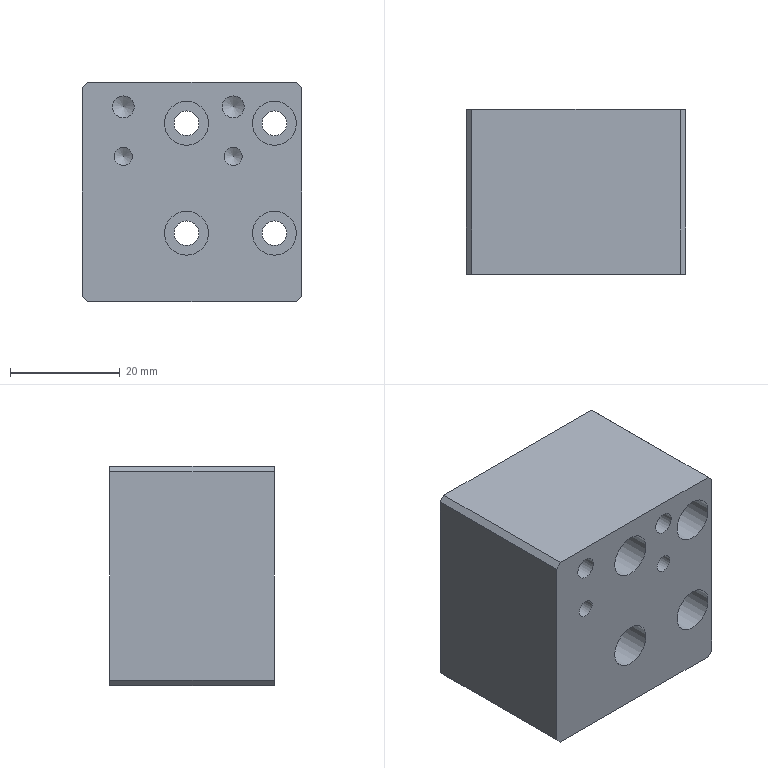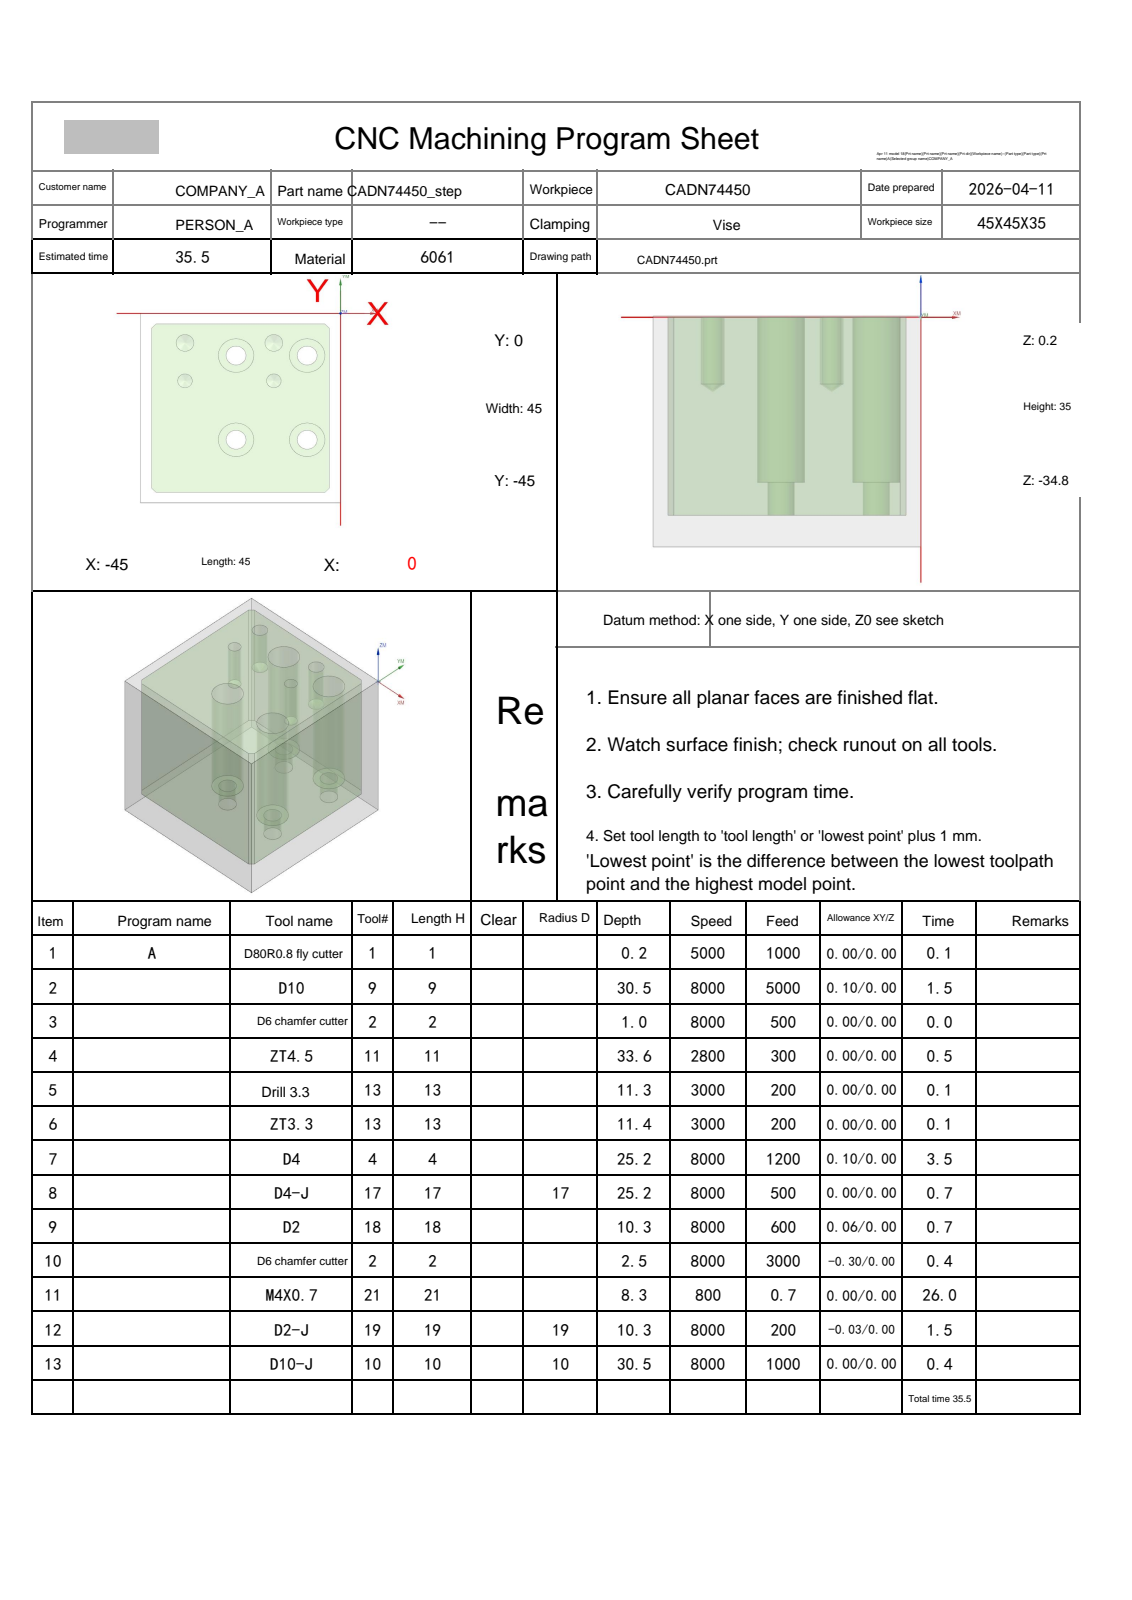NC program | NX | posted by the shop | part box 40 x 30 x 40 mm
Whole program, first 1137 of 1731 lines:
%
O0001
(Machine time: 61.34 MIN)
(===Total Tool:11===)
(T1=D80R0.8 fly cutter D=80.  R=0.8  D-  H01 Z=0.    )
(T9=D10     D=10.  R=0.   D-  H09 Z=-30.3 )
(T2=D6 chamfer cutter   D=6.   R=0.   D-  H02 Z=-2.3  )
(T11=ZT4.5  D=4.5  DR_a=118 D-  H11 Z=-33.35)
(T13=Drill 3.3  D=3.3  DR_a=118 D-  H13 Z=-11.2 )
(T4=D4      D=4.   R=0.   D-  H04 Z=-25.  )
(T17=D4-J   D=4.   R=0.   D17 H17 Z=-25.  )
(T18=D2     D=2.   R=0.   D-  H18 Z=-10.1 )
(T21=M4X0.7 D=3.3  DR_a=180 D-  H21 Z=-8.1  )
(T19=D2-J   D=2.   R=0.   D19 H19 Z=-10.1 )
(T10=D10-J  D=10.  R=0.   D10 H10 Z=-30.3 )
G80 G90 G17 G49 G40
G91 G28 Z0
M01
N1 T01 M06
(D80R0.8 fly cutter  D=80. R=0.8 H=01 ce=0.00 di=0.00)
G00 G90 G54 X-22.5 Y-87.5 M03 S5000
G43 H01 Z20.
M08
Z2.
G01 Z0.0 F1000.
Y-82.5
Y37.5
Y42.5
Z2.
G00 Z20.
G91 G28 Z0.0
M05
M09
G91 G28 Z0.0
M01
N2 T09 M06
(D10  D=10. R=0. H=09 ce=0.10 di=0.00)
G00 G90 G54 X-22.5 Y-47.6 M03 S8000
G43 H09 Z20.
M08
Z.5
G01 X-41.5 Z.421 F5000.
G02 X-45.106 Y-46.106 Z.404 I0.0 J5.1
G01 X-46.106 Y-45.106 Z.398
G02 X-47.6 Y-41.5 Z.382 I3.606 J3.606
G01 Y-3.5 Z.223
G02 X-46.106 Y.106 Z.207 I5.1 J0.0
G01 X-45.106 Y1.106 Z.201
G02 X-41.5 Y2.6 Z.184 I3.606 J-3.606
G01 X-3.5 Z.026
G02 X.106 Y1.106 Z.009 I0.0 J-5.1
G01 X1.106 Y.106 Z.003
G02 X2.6 Y-3.5 Z-.013 I-3.606 J-3.606
G01 Y-41.5 Z-.171
G02 X1.106 Y-45.106 Z-.188 I-5.1 J0.0
G01 X.106 Y-46.106 Z-.194
G02 X-3.5 Y-47.6 Z-.211 I-3.606 J3.606
G01 X-41.5 Z-.369
G02 X-45.106 Y-46.106 Z-.386 I0.0 J5.1
G01 X-46.106 Y-45.106 Z-.391
G02 X-47.6 Y-41.5 Z-.408 I3.606 J3.606
G01 Y-3.5 Z-.566
G02 X-46.106 Y.106 Z-.583 I5.1 J0.0
G01 X-45.106 Y1.106 Z-.589
G02 X-41.5 Y2.6 Z-.606 I3.606 J-3.606
G01 X-3.5 Z-.764
G02 X.106 Y1.106 Z-.78 I0.0 J-5.1
G01 X1.106 Y.106 Z-.786
G02 X2.6 Y-3.5 Z-.803 I-3.606 J-3.606
G01 Y-41.5 Z-.961
G02 X1.106 Y-45.106 Z-.978 I-5.1 J0.0
G01 X.106 Y-46.106 Z-.984
G02 X-3.5 Y-47.6 Z-1. I-3.606 J3.606
G01 X-41.5 Z-1.159
G02 X-45.106 Y-46.106 Z-1.175 I0.0 J5.1
G01 X-46.106 Y-45.106 Z-1.181
G02 X-47.6 Y-41.5 Z-1.198 I3.606 J3.606
G01 Y-3.5 Z-1.356
G02 X-46.106 Y.106 Z-1.373 I5.1 J0.0
G01 X-45.106 Y1.106 Z-1.379
G02 X-41.5 Y2.6 Z-1.395 I3.606 J-3.606
G01 X-3.5 Z-1.553
G02 X.106 Y1.106 Z-1.57 I0.0 J-5.1
G01 X1.106 Y.106 Z-1.576
G02 X2.6 Y-3.5 Z-1.593 I-3.606 J-3.606
G01 Y-41.5 Z-1.751
G02 X1.106 Y-45.106 Z-1.768 I-5.1 J0.0
G01 X.106 Y-46.106 Z-1.773
G02 X-3.5 Y-47.6 Z-1.79 I-3.606 J3.606
G01 X-41.5 Z-1.948
G02 X-45.106 Y-46.106 Z-1.965 I0.0 J5.1
G01 X-46.106 Y-45.106 Z-1.971
G02 X-47.6 Y-41.5 Z-1.988 I3.606 J3.606
G01 Y-3.5 Z-2.146
G02 X-46.106 Y.106 Z-2.162 I5.1 J0.0
G01 X-45.106 Y1.106 Z-2.168
G02 X-41.5 Y2.6 Z-2.185 I3.606 J-3.606
G01 X-3.5 Z-2.343
G02 X.106 Y1.106 Z-2.36 I0.0 J-5.1
G01 X1.106 Y.106 Z-2.366
G02 X2.6 Y-3.5 Z-2.382 I-3.606 J-3.606
G01 Y-41.5 Z-2.541
G02 X1.106 Y-45.106 Z-2.557 I-5.1 J0.0
G01 X.106 Y-46.106 Z-2.563
G02 X-3.5 Y-47.6 Z-2.58 I-3.606 J3.606
G01 X-41.5 Z-2.738
G02 X-45.106 Y-46.106 Z-2.755 I0.0 J5.1
G01 X-46.106 Y-45.106 Z-2.761
G02 X-47.6 Y-41.5 Z-2.777 I3.606 J3.606
G01 Y-3.5 Z-2.936
G02 X-46.106 Y.106 Z-2.952 I5.1 J0.0
G01 X-45.106 Y1.106 Z-2.958
G02 X-41.5 Y2.6 Z-2.975 I3.606 J-3.606
G01 X-3.5 Z-3.133
G02 X.106 Y1.106 Z-3.15 I0.0 J-5.1
G01 X1.106 Y.106 Z-3.156
G02 X2.6 Y-3.5 Z-3.172 I-3.606 J-3.606
G01 Y-41.5 Z-3.33
G02 X1.106 Y-45.106 Z-3.347 I-5.1 J0.0
G01 X.106 Y-46.106 Z-3.353
G02 X-3.5 Y-47.6 Z-3.37 I-3.606 J3.606
G01 X-41.5 Z-3.528
G02 X-45.106 Y-46.106 Z-3.544 I0.0 J5.1
G01 X-46.106 Y-45.106 Z-3.55
G02 X-47.6 Y-41.5 Z-3.567 I3.606 J3.606
G01 Y-3.5 Z-3.725
G02 X-46.106 Y.106 Z-3.742 I5.1 J0.0
G01 X-45.106 Y1.106 Z-3.748
G02 X-41.5 Y2.6 Z-3.764 I3.606 J-3.606
G01 X-3.5 Z-3.923
G02 X.106 Y1.106 Z-3.939 I0.0 J-5.1
G01 X1.106 Y.106 Z-3.945
G02 X2.6 Y-3.5 Z-3.962 I-3.606 J-3.606
G01 Y-41.5 Z-4.12
G02 X1.106 Y-45.106 Z-4.137 I-5.1 J0.0
G01 X.106 Y-46.106 Z-4.143
G02 X-3.5 Y-47.6 Z-4.159 I-3.606 J3.606
G01 X-41.5 Z-4.318
G02 X-45.106 Y-46.106 Z-4.334 I0.0 J5.1
G01 X-46.106 Y-45.106 Z-4.34
G02 X-47.6 Y-41.5 Z-4.357 I3.606 J3.606
G01 Y-3.5 Z-4.515
G02 X-46.106 Y.106 Z-4.532 I5.1 J0.0
G01 X-45.106 Y1.106 Z-4.538
G02 X-41.5 Y2.6 Z-4.554 I3.606 J-3.606
G01 X-3.5 Z-4.712
G02 X.106 Y1.106 Z-4.729 I0.0 J-5.1
G01 X1.106 Y.106 Z-4.735
G02 X2.6 Y-3.5 Z-4.752 I-3.606 J-3.606
G01 Y-41.5 Z-4.91
G02 X1.106 Y-45.106 Z-4.927 I-5.1 J0.0
G01 X.106 Y-46.106 Z-4.932
G02 X-3.5 Y-47.6 Z-4.949 I-3.606 J3.606
G01 X-41.5 Z-5.107
G02 X-45.106 Y-46.106 Z-5.124 I0.0 J5.1
G01 X-46.106 Y-45.106 Z-5.13
G02 X-47.6 Y-41.5 Z-5.147 I3.606 J3.606
G01 Y-3.5 Z-5.305
G02 X-46.106 Y.106 Z-5.321 I5.1 J0.0
G01 X-45.106 Y1.106 Z-5.327
G02 X-41.5 Y2.6 Z-5.344 I3.606 J-3.606
G01 X-3.5 Z-5.502
G02 X.106 Y1.106 Z-5.519 I0.0 J-5.1
G01 X1.106 Y.106 Z-5.525
G02 X2.6 Y-3.5 Z-5.541 I-3.606 J-3.606
G01 Y-41.5 Z-5.7
G02 X1.106 Y-45.106 Z-5.716 I-5.1 J0.0
G01 X.106 Y-46.106 Z-5.722
G02 X-3.5 Y-47.6 Z-5.739 I-3.606 J3.606
G01 X-41.5 Z-5.897
G02 X-45.106 Y-46.106 Z-5.914 I0.0 J5.1
G01 X-46.106 Y-45.106 Z-5.92
G02 X-47.6 Y-41.5 Z-5.936 I3.606 J3.606
G01 Y-3.5 Z-6.094
G02 X-46.106 Y.106 Z-6.111 I5.1 J0.0
G01 X-45.106 Y1.106 Z-6.117
G02 X-41.5 Y2.6 Z-6.134 I3.606 J-3.606
G01 X-3.5 Z-6.292
G02 X.106 Y1.106 Z-6.309 I0.0 J-5.1
G01 X1.106 Y.106 Z-6.314
G02 X2.6 Y-3.5 Z-6.331 I-3.606 J-3.606
G01 Y-41.5 Z-6.489
G02 X1.106 Y-45.106 Z-6.506 I-5.1 J0.0
G01 X.106 Y-46.106 Z-6.512
G02 X-3.5 Y-47.6 Z-6.529 I-3.606 J3.606
G01 X-41.5 Z-6.687
G02 X-45.106 Y-46.106 Z-6.703 I0.0 J5.1
G01 X-46.106 Y-45.106 Z-6.709
G02 X-47.6 Y-41.5 Z-6.726 I3.606 J3.606
G01 Y-3.5 Z-6.884
G02 X-46.106 Y.106 Z-6.901 I5.1 J0.0
G01 X-45.106 Y1.106 Z-6.907
G02 X-41.5 Y2.6 Z-6.923 I3.606 J-3.606
G01 X-3.5 Z-7.082
G02 X.106 Y1.106 Z-7.098 I0.0 J-5.1
G01 X1.106 Y.106 Z-7.104
G02 X2.6 Y-3.5 Z-7.121 I-3.606 J-3.606
G01 Y-41.5 Z-7.279
G02 X1.106 Y-45.106 Z-7.296 I-5.1 J0.0
G01 X.106 Y-46.106 Z-7.302
G02 X-3.5 Y-47.6 Z-7.318 I-3.606 J3.606
G01 X-41.5 Z-7.477
G02 X-45.106 Y-46.106 Z-7.493 I0.0 J5.1
G01 X-46.106 Y-45.106 Z-7.499
G02 X-47.6 Y-41.5 Z-7.516 I3.606 J3.606
G01 Y-3.5 Z-7.674
G02 X-46.106 Y.106 Z-7.691 I5.1 J0.0
G01 X-45.106 Y1.106 Z-7.697
G02 X-41.5 Y2.6 Z-7.713 I3.606 J-3.606
G01 X-3.5 Z-7.871
G02 X.106 Y1.106 Z-7.888 I0.0 J-5.1
G01 X1.106 Y.106 Z-7.894
G02 X2.6 Y-3.5 Z-7.911 I-3.606 J-3.606
G01 Y-41.5 Z-8.069
G02 X1.106 Y-45.106 Z-8.086 I-5.1 J0.0
G01 X.106 Y-46.106 Z-8.091
G02 X-3.5 Y-47.6 Z-8.108 I-3.606 J3.606
G01 X-41.5 Z-8.266
G02 X-45.106 Y-46.106 Z-8.283 I0.0 J5.1
G01 X-46.106 Y-45.106 Z-8.289
G02 X-47.6 Y-41.5 Z-8.306 I3.606 J3.606
G01 Y-3.5 Z-8.464
G02 X-46.106 Y.106 Z-8.48 I5.1 J0.0
G01 X-45.106 Y1.106 Z-8.486
G02 X-41.5 Y2.6 Z-8.503 I3.606 J-3.606
G01 X-3.5 Z-8.661
G02 X.106 Y1.106 Z-8.678 I0.0 J-5.1
G01 X1.106 Y.106 Z-8.684
G02 X2.6 Y-3.5 Z-8.7 I-3.606 J-3.606
G01 Y-41.5 Z-8.859
G02 X1.106 Y-45.106 Z-8.875 I-5.1 J0.0
G01 X.106 Y-46.106 Z-8.881
G02 X-3.5 Y-47.6 Z-8.898 I-3.606 J3.606
G01 X-41.5 Z-9.056
G02 X-45.106 Y-46.106 Z-9.073 I0.0 J5.1
G01 X-46.106 Y-45.106 Z-9.079
G02 X-47.6 Y-41.5 Z-9.095 I3.606 J3.606
G01 Y-3.5 Z-9.253
G02 X-46.106 Y.106 Z-9.27 I5.1 J0.0
G01 X-45.106 Y1.106 Z-9.276
G02 X-41.5 Y2.6 Z-9.293 I3.606 J-3.606
G01 X-3.5 Z-9.451
G02 X.106 Y1.106 Z-9.468 I0.0 J-5.1
G01 X1.106 Y.106 Z-9.473
G02 X2.6 Y-3.5 Z-9.49 I-3.606 J-3.606
G01 Y-41.5 Z-9.648
G02 X1.106 Y-45.106 Z-9.665 I-5.1 J0.0
G01 X.106 Y-46.106 Z-9.671
G02 X-3.5 Y-47.6 Z-9.688 I-3.606 J3.606
G01 X-41.5 Z-9.846
G02 X-45.106 Y-46.106 Z-9.862 I0.0 J5.1
G01 X-46.106 Y-45.106 Z-9.868
G02 X-47.6 Y-41.5 Z-9.885 I3.606 J3.606
G01 Y-3.5 Z-10.043
G02 X-46.106 Y.106 Z-10.06 I5.1 J0.0
G01 X-45.106 Y1.106 Z-10.066
G02 X-41.5 Y2.6 Z-10.082 I3.606 J-3.606
G01 X-3.5 Z-10.241
G02 X.106 Y1.106 Z-10.257 I0.0 J-5.1
G01 X1.106 Y.106 Z-10.263
G02 X2.6 Y-3.5 Z-10.28 I-3.606 J-3.606
G01 Y-41.5 Z-10.438
G02 X1.106 Y-45.106 Z-10.455 I-5.1 J0.0
G01 X.106 Y-46.106 Z-10.461
G02 X-3.5 Y-47.6 Z-10.477 I-3.606 J3.606
G01 X-41.5 Z-10.636
G02 X-45.106 Y-46.106 Z-10.652 I0.0 J5.1
G01 X-46.106 Y-45.106 Z-10.658
G02 X-47.6 Y-41.5 Z-10.675 I3.606 J3.606
G01 Y-3.5 Z-10.833
G02 X-46.106 Y.106 Z-10.85 I5.1 J0.0
G01 X-45.106 Y1.106 Z-10.856
G02 X-41.5 Y2.6 Z-10.872 I3.606 J-3.606
G01 X-3.5 Z-11.03
G02 X.106 Y1.106 Z-11.047 I0.0 J-5.1
G01 X1.106 Y.106 Z-11.053
G02 X2.6 Y-3.5 Z-11.07 I-3.606 J-3.606
G01 Y-41.5 Z-11.228
G02 X1.106 Y-45.106 Z-11.244 I-5.1 J0.0
G01 X.106 Y-46.106 Z-11.25
G02 X-3.5 Y-47.6 Z-11.267 I-3.606 J3.606
G01 X-41.5 Z-11.425
G02 X-45.106 Y-46.106 Z-11.442 I0.0 J5.1
G01 X-46.106 Y-45.106 Z-11.448
G02 X-47.6 Y-41.5 Z-11.464 I3.606 J3.606
G01 Y-3.5 Z-11.623
G02 X-46.106 Y.106 Z-11.639 I5.1 J0.0
G01 X-45.106 Y1.106 Z-11.645
G02 X-41.5 Y2.6 Z-11.662 I3.606 J-3.606
G01 X-3.5 Z-11.82
G02 X.106 Y1.106 Z-11.837 I0.0 J-5.1
G01 X1.106 Y.106 Z-11.843
G02 X2.6 Y-3.5 Z-11.859 I-3.606 J-3.606
G01 Y-41.5 Z-12.018
G02 X1.106 Y-45.106 Z-12.034 I-5.1 J0.0
G01 X.106 Y-46.106 Z-12.04
G02 X-3.5 Y-47.6 Z-12.057 I-3.606 J3.606
G01 X-41.5 Z-12.215
G02 X-45.106 Y-46.106 Z-12.232 I0.0 J5.1
G01 X-46.106 Y-45.106 Z-12.238
G02 X-47.6 Y-41.5 Z-12.254 I3.606 J3.606
G01 Y-3.5 Z-12.412
G02 X-46.106 Y.106 Z-12.429 I5.1 J0.0
G01 X-45.106 Y1.106 Z-12.435
G02 X-41.5 Y2.6 Z-12.452 I3.606 J-3.606
G01 X-3.5 Z-12.61
G02 X.106 Y1.106 Z-12.627 I0.0 J-5.1
G01 X1.106 Y.106 Z-12.632
G02 X2.6 Y-3.5 Z-12.649 I-3.606 J-3.606
G01 Y-41.5 Z-12.807
G02 X1.106 Y-45.106 Z-12.824 I-5.1 J0.0
G01 X.106 Y-46.106 Z-12.83
G02 X-3.5 Y-47.6 Z-12.847 I-3.606 J3.606
G01 X-41.5 Z-13.005
G02 X-45.106 Y-46.106 Z-13.021 I0.0 J5.1
G01 X-46.106 Y-45.106 Z-13.027
G02 X-47.6 Y-41.5 Z-13.044 I3.606 J3.606
G01 Y-3.5 Z-13.202
G02 X-46.106 Y.106 Z-13.219 I5.1 J0.0
G01 X-45.106 Y1.106 Z-13.225
G02 X-41.5 Y2.6 Z-13.241 I3.606 J-3.606
G01 X-3.5 Z-13.4
G02 X.106 Y1.106 Z-13.416 I0.0 J-5.1
G01 X1.106 Y.106 Z-13.422
G02 X2.6 Y-3.5 Z-13.439 I-3.606 J-3.606
G01 Y-41.5 Z-13.597
G02 X1.106 Y-45.106 Z-13.614 I-5.1 J0.0
G01 X.106 Y-46.106 Z-13.62
G02 X-3.5 Y-47.6 Z-13.636 I-3.606 J3.606
G01 X-41.5 Z-13.794
G02 X-45.106 Y-46.106 Z-13.811 I0.0 J5.1
G01 X-46.106 Y-45.106 Z-13.817
G02 X-47.6 Y-41.5 Z-13.834 I3.606 J3.606
G01 Y-3.5 Z-13.992
G02 X-46.106 Y.106 Z-14.009 I5.1 J0.0
G01 X-45.106 Y1.106 Z-14.014
G02 X-41.5 Y2.6 Z-14.031 I3.606 J-3.606
G01 X-3.5 Z-14.189
G02 X.106 Y1.106 Z-14.206 I0.0 J-5.1
G01 X1.106 Y.106 Z-14.212
G02 X2.6 Y-3.5 Z-14.229 I-3.606 J-3.606
G01 Y-41.5 Z-14.387
G02 X1.106 Y-45.106 Z-14.403 I-5.1 J0.0
G01 X.106 Y-46.106 Z-14.409
G02 X-3.5 Y-47.6 Z-14.426 I-3.606 J3.606
G01 X-41.5 Z-14.584
G02 X-45.106 Y-46.106 Z-14.601 I0.0 J5.1
G01 X-46.106 Y-45.106 Z-14.607
G02 X-47.6 Y-41.5 Z-14.623 I3.606 J3.606
G01 Y-3.5 Z-14.782
G02 X-46.106 Y.106 Z-14.798 I5.1 J0.0
G01 X-45.106 Y1.106 Z-14.804
G02 X-41.5 Y2.6 Z-14.821 I3.606 J-3.606
G01 X-3.5 Z-14.979
G02 X.106 Y1.106 Z-14.996 I0.0 J-5.1
G01 X1.106 Y.106 Z-15.002
G02 X2.6 Y-3.5 Z-15.018 I-3.606 J-3.606
G01 Y-41.5 Z-15.177
G02 X1.106 Y-45.106 Z-15.193 I-5.1 J0.0
G01 X.106 Y-46.106 Z-15.199
G02 X-3.5 Y-47.6 Z-15.216 I-3.606 J3.606
G01 X-41.5 Z-15.374
G02 X-45.106 Y-46.106 Z-15.391 I0.0 J5.1
G01 X-46.106 Y-45.106 Z-15.397
G02 X-47.6 Y-41.5 Z-15.413 I3.606 J3.606
G01 Y-3.5 Z-15.571
G02 X-46.106 Y.106 Z-15.588 I5.1 J0.0
G01 X-45.106 Y1.106 Z-15.594
G02 X-41.5 Y2.6 Z-15.611 I3.606 J-3.606
G01 X-3.5 Z-15.769
G02 X.106 Y1.106 Z-15.786 I0.0 J-5.1
G01 X1.106 Y.106 Z-15.791
G02 X2.6 Y-3.5 Z-15.808 I-3.606 J-3.606
G01 Y-41.5 Z-15.966
G02 X1.106 Y-45.106 Z-15.983 I-5.1 J0.0
G01 X.106 Y-46.106 Z-15.989
G02 X-3.5 Y-47.6 Z-16.006 I-3.606 J3.606
G01 X-41.5 Z-16.164
G02 X-45.106 Y-46.106 Z-16.18 I0.0 J5.1
G01 X-46.106 Y-45.106 Z-16.186
G02 X-47.6 Y-41.5 Z-16.203 I3.606 J3.606
G01 Y-3.5 Z-16.361
G02 X-46.106 Y.106 Z-16.378 I5.1 J0.0
G01 X-45.106 Y1.106 Z-16.384
G02 X-41.5 Y2.6 Z-16.4 I3.606 J-3.606
G01 X-3.5 Z-16.559
G02 X.106 Y1.106 Z-16.575 I0.0 J-5.1
G01 X1.106 Y.106 Z-16.581
G02 X2.6 Y-3.5 Z-16.598 I-3.606 J-3.606
G01 Y-41.5 Z-16.756
G02 X1.106 Y-45.106 Z-16.773 I-5.1 J0.0
G01 X.106 Y-46.106 Z-16.779
G02 X-3.5 Y-47.6 Z-16.795 I-3.606 J3.606
G01 X-41.5 Z-16.953
G02 X-45.106 Y-46.106 Z-16.97 I0.0 J5.1
G01 X-46.106 Y-45.106 Z-16.976
G02 X-47.6 Y-41.5 Z-16.993 I3.606 J3.606
G01 Y-3.5 Z-17.151
G02 X-46.106 Y.106 Z-17.168 I5.1 J0.0
G01 X-45.106 Y1.106 Z-17.173
G02 X-41.5 Y2.6 Z-17.19 I3.606 J-3.606
G01 X-3.5 Z-17.348
G02 X.106 Y1.106 Z-17.365 I0.0 J-5.1
G01 X1.106 Y.106 Z-17.371
G02 X2.6 Y-3.5 Z-17.388 I-3.606 J-3.606
G01 Y-41.5 Z-17.546
G02 X1.106 Y-45.106 Z-17.562 I-5.1 J0.0
G01 X.106 Y-46.106 Z-17.568
G02 X-3.5 Y-47.6 Z-17.585 I-3.606 J3.606
G01 X-41.5 Z-17.743
G02 X-45.106 Y-46.106 Z-17.76 I0.0 J5.1
G01 X-46.106 Y-45.106 Z-17.766
G02 X-47.6 Y-41.5 Z-17.782 I3.606 J3.606
G01 Y-3.5 Z-17.941
G02 X-46.106 Y.106 Z-17.957 I5.1 J0.0
G01 X-45.106 Y1.106 Z-17.963
G02 X-41.5 Y2.6 Z-17.98 I3.606 J-3.606
G01 X-3.5 Z-18.138
G02 X.106 Y1.106 Z-18.155 I0.0 J-5.1
G01 X1.106 Y.106 Z-18.161
G02 X2.6 Y-3.5 Z-18.177 I-3.606 J-3.606
G01 Y-41.5 Z-18.336
G02 X1.106 Y-45.106 Z-18.352 I-5.1 J0.0
G01 X.106 Y-46.106 Z-18.358
G02 X-3.5 Y-47.6 Z-18.375 I-3.606 J3.606
G01 X-41.5 Z-18.533
G02 X-45.106 Y-46.106 Z-18.55 I0.0 J5.1
G01 X-46.106 Y-45.106 Z-18.556
G02 X-47.6 Y-41.5 Z-18.572 I3.606 J3.606
G01 Y-3.5 Z-18.73
G02 X-46.106 Y.106 Z-18.747 I5.1 J0.0
G01 X-45.106 Y1.106 Z-18.753
G02 X-41.5 Y2.6 Z-18.77 I3.606 J-3.606
G01 X-3.5 Z-18.928
G02 X.106 Y1.106 Z-18.944 I0.0 J-5.1
G01 X1.106 Y.106 Z-18.95
G02 X2.6 Y-3.5 Z-18.967 I-3.606 J-3.606
G01 Y-41.5 Z-19.125
G02 X1.106 Y-45.106 Z-19.142 I-5.1 J0.0
G01 X.106 Y-46.106 Z-19.148
G02 X-3.5 Y-47.6 Z-19.164 I-3.606 J3.606
G01 X-41.5 Z-19.323
G02 X-45.106 Y-46.106 Z-19.339 I0.0 J5.1
G01 X-46.106 Y-45.106 Z-19.345
G02 X-47.6 Y-41.5 Z-19.362 I3.606 J3.606
G01 Y-3.5 Z-19.52
G02 X-46.106 Y.106 Z-19.537 I5.1 J0.0
G01 X-45.106 Y1.106 Z-19.543
G02 X-41.5 Y2.6 Z-19.559 I3.606 J-3.606
G01 X-3.5 Z-19.718
G02 X.106 Y1.106 Z-19.734 I0.0 J-5.1
G01 X1.106 Y.106 Z-19.74
G02 X2.6 Y-3.5 Z-19.757 I-3.606 J-3.606
G01 Y-41.5 Z-19.915
G02 X1.106 Y-45.106 Z-19.932 I-5.1 J0.0
G01 X.106 Y-46.106 Z-19.938
G02 X-3.5 Y-47.6 Z-19.954 I-3.606 J3.606
G01 X-41.5 Z-20.112
G02 X-45.106 Y-46.106 Z-20.129 I0.0 J5.1
G01 X-46.106 Y-45.106 Z-20.135
G02 X-47.6 Y-41.5 Z-20.152 I3.606 J3.606
G01 Y-3.5 Z-20.31
G02 X-46.106 Y.106 Z-20.327 I5.1 J0.0
G01 X-45.106 Y1.106 Z-20.332
G02 X-41.5 Y2.6 Z-20.349 I3.606 J-3.606
G01 X-3.5 Z-20.507
G02 X.106 Y1.106 Z-20.524 I0.0 J-5.1
G01 X1.106 Y.106 Z-20.53
G02 X2.6 Y-3.5 Z-20.547 I-3.606 J-3.606
G01 Y-41.5 Z-20.705
G02 X1.106 Y-45.106 Z-20.721 I-5.1 J0.0
G01 X.106 Y-46.106 Z-20.727
G02 X-3.5 Y-47.6 Z-20.744 I-3.606 J3.606
G01 X-41.5 Z-20.902
G02 X-45.106 Y-46.106 Z-20.919 I0.0 J5.1
G01 X-46.106 Y-45.106 Z-20.925
G02 X-47.6 Y-41.5 Z-20.941 I3.606 J3.606
G01 Y-3.5 Z-21.1
G02 X-46.106 Y.106 Z-21.116 I5.1 J0.0
G01 X-45.106 Y1.106 Z-21.122
G02 X-41.5 Y2.6 Z-21.139 I3.606 J-3.606
G01 X-3.5 Z-21.297
G02 X.106 Y1.106 Z-21.314 I0.0 J-5.1
G01 X1.106 Y.106 Z-21.32
G02 X2.6 Y-3.5 Z-21.336 I-3.606 J-3.606
G01 Y-41.5 Z-21.494
G02 X1.106 Y-45.106 Z-21.511 I-5.1 J0.0
G01 X.106 Y-46.106 Z-21.517
G02 X-3.5 Y-47.6 Z-21.534 I-3.606 J3.606
G01 X-41.5 Z-21.692
G02 X-45.106 Y-46.106 Z-21.709 I0.0 J5.1
G01 X-46.106 Y-45.106 Z-21.714
G02 X-47.6 Y-41.5 Z-21.731 I3.606 J3.606
G01 Y-3.5 Z-21.889
G02 X-46.106 Y.106 Z-21.906 I5.1 J0.0
G01 X-45.106 Y1.106 Z-21.912
G02 X-41.5 Y2.6 Z-21.929 I3.606 J-3.606
G01 X-3.5 Z-22.087
G02 X.106 Y1.106 Z-22.103 I0.0 J-5.1
G01 X1.106 Y.106 Z-22.109
G02 X2.6 Y-3.5 Z-22.126 I-3.606 J-3.606
G01 Y-41.5 Z-22.284
G02 X1.106 Y-45.106 Z-22.301 I-5.1 J0.0
G01 X.106 Y-46.106 Z-22.307
G02 X-3.5 Y-47.6 Z-22.323 I-3.606 J3.606
G01 X-41.5 Z-22.482
G02 X-45.106 Y-46.106 Z-22.498 I0.0 J5.1
G01 X-46.106 Y-45.106 Z-22.504
G02 X-47.6 Y-41.5 Z-22.521 I3.606 J3.606
G01 Y-3.5 Z-22.679
G02 X-46.106 Y.106 Z-22.696 I5.1 J0.0
G01 X-45.106 Y1.106 Z-22.702
G02 X-41.5 Y2.6 Z-22.718 I3.606 J-3.606
G01 X-3.5 Z-22.877
G02 X.106 Y1.106 Z-22.893 I0.0 J-5.1
G01 X1.106 Y.106 Z-22.899
G02 X2.6 Y-3.5 Z-22.916 I-3.606 J-3.606
G01 Y-41.5 Z-23.074
G02 X1.106 Y-45.106 Z-23.091 I-5.1 J0.0
G01 X.106 Y-46.106 Z-23.097
G02 X-3.5 Y-47.6 Z-23.113 I-3.606 J3.606
G01 X-41.5 Z-23.271
G02 X-45.106 Y-46.106 Z-23.288 I0.0 J5.1
G01 X-46.106 Y-45.106 Z-23.294
G02 X-47.6 Y-41.5 Z-23.311 I3.606 J3.606
G01 Y-3.5 Z-23.469
G02 X-46.106 Y.106 Z-23.486 I5.1 J0.0
G01 X-45.106 Y1.106 Z-23.491
G02 X-41.5 Y2.6 Z-23.508 I3.606 J-3.606
G01 X-3.5 Z-23.666
G02 X.106 Y1.106 Z-23.683 I0.0 J-5.1
G01 X1.106 Y.106 Z-23.689
G02 X2.6 Y-3.5 Z-23.706 I-3.606 J-3.606
G01 Y-41.5 Z-23.864
G02 X1.106 Y-45.106 Z-23.88 I-5.1 J0.0
G01 X.106 Y-46.106 Z-23.886
G02 X-3.5 Y-47.6 Z-23.903 I-3.606 J3.606
G01 X-41.5 Z-24.061
G02 X-45.106 Y-46.106 Z-24.078 I0.0 J5.1
G01 X-46.106 Y-45.106 Z-24.084
G02 X-47.6 Y-41.5 Z-24.1 I3.606 J3.606
G01 Y-3.5 Z-24.259
G02 X-46.106 Y.106 Z-24.275 I5.1 J0.0
G01 X-45.106 Y1.106 Z-24.281
G02 X-41.5 Y2.6 Z-24.298 I3.606 J-3.606
G01 X-3.5 Z-24.456
G02 X.106 Y1.106 Z-24.473 I0.0 J-5.1
G01 X1.106 Y.106 Z-24.479
G02 X2.6 Y-3.5 Z-24.495 I-3.606 J-3.606
G01 Y-41.5 Z-24.653
G02 X1.106 Y-45.106 Z-24.67 I-5.1 J0.0
G01 X.106 Y-46.106 Z-24.676
G02 X-3.5 Y-47.6 Z-24.693 I-3.606 J3.606
G01 X-41.5 Z-24.851
G02 X-45.106 Y-46.106 Z-24.868 I0.0 J5.1
G01 X-46.106 Y-45.106 Z-24.873
G02 X-47.6 Y-41.5 Z-24.89 I3.606 J3.606
G01 Y-3.5 Z-25.048
G02 X-46.106 Y.106 Z-25.065 I5.1 J0.0
G01 X-45.106 Y1.106 Z-25.071
G02 X-41.5 Y2.6 Z-25.088 I3.606 J-3.606
G01 X-3.5 Z-25.246
G02 X.106 Y1.106 Z-25.262 I0.0 J-5.1
G01 X1.106 Y.106 Z-25.268
G02 X2.6 Y-3.5 Z-25.285 I-3.606 J-3.606
G01 Y-41.5 Z-25.443
G02 X1.106 Y-45.106 Z-25.46 I-5.1 J0.0
G01 X.106 Y-46.106 Z-25.466
G02 X-3.5 Y-47.6 Z-25.482 I-3.606 J3.606
G01 X-41.5 Z-25.641
G02 X-45.106 Y-46.106 Z-25.657 I0.0 J5.1
G01 X-46.106 Y-45.106 Z-25.663
G02 X-47.6 Y-41.5 Z-25.68 I3.606 J3.606
G01 Y-3.5 Z-25.838
G02 X-46.106 Y.106 Z-25.855 I5.1 J0.0
G01 X-45.106 Y1.106 Z-25.861
G02 X-41.5 Y2.6 Z-25.877 I3.606 J-3.606
G01 X-3.5 Z-26.036
G02 X.106 Y1.106 Z-26.052 I0.0 J-5.1
G01 X1.106 Y.106 Z-26.058
G02 X2.6 Y-3.5 Z-26.075 I-3.606 J-3.606
G01 Y-41.5 Z-26.233
G02 X1.106 Y-45.106 Z-26.25 I-5.1 J0.0
G01 X.106 Y-46.106 Z-26.256
G02 X-3.5 Y-47.6 Z-26.272 I-3.606 J3.606
G01 X-41.5 Z-26.43
G02 X-45.106 Y-46.106 Z-26.447 I0.0 J5.1
G01 X-46.106 Y-45.106 Z-26.453
G02 X-47.6 Y-41.5 Z-26.47 I3.606 J3.606
G01 Y-3.5 Z-26.628
G02 X-46.106 Y.106 Z-26.644 I5.1 J0.0
G01 X-45.106 Y1.106 Z-26.65
G02 X-41.5 Y2.6 Z-26.667 I3.606 J-3.606
G01 X-3.5 Z-26.825
G02 X.106 Y1.106 Z-26.842 I0.0 J-5.1
G01 X1.106 Y.106 Z-26.848
G02 X2.6 Y-3.5 Z-26.864 I-3.606 J-3.606
G01 Y-41.5 Z-27.023
G02 X1.106 Y-45.106 Z-27.039 I-5.1 J0.0
G01 X.106 Y-46.106 Z-27.045
G02 X-3.5 Y-47.6 Z-27.062 I-3.606 J3.606
G01 X-41.5 Z-27.22
G02 X-45.106 Y-46.106 Z-27.237 I0.0 J5.1
G01 X-46.106 Y-45.106 Z-27.243
G02 X-47.6 Y-41.5 Z-27.259 I3.606 J3.606
G01 Y-3.5 Z-27.418
G02 X-46.106 Y.106 Z-27.434 I5.1 J0.0
G01 X-45.106 Y1.106 Z-27.44
G02 X-41.5 Y2.6 Z-27.457 I3.606 J-3.606
G01 X-3.5 Z-27.615
G02 X.106 Y1.106 Z-27.632 I0.0 J-5.1
G01 X1.106 Y.106 Z-27.638
G02 X2.6 Y-3.5 Z-27.654 I-3.606 J-3.606
G01 Y-41.5 Z-27.812
G02 X1.106 Y-45.106 Z-27.829 I-5.1 J0.0
G01 X.106 Y-46.106 Z-27.835
G02 X-3.5 Y-47.6 Z-27.852 I-3.606 J3.606
G01 X-41.5 Z-28.01
G02 X-45.106 Y-46.106 Z-28.027 I0.0 J5.1
G01 X-46.106 Y-45.106 Z-28.032
G02 X-47.6 Y-41.5 Z-28.049 I3.606 J3.606
G01 Y-3.5 Z-28.207
G02 X-46.106 Y.106 Z-28.224 I5.1 J0.0
G01 X-45.106 Y1.106 Z-28.23
G02 X-41.5 Y2.6 Z-28.247 I3.606 J-3.606
G01 X-3.5 Z-28.405
G02 X.106 Y1.106 Z-28.421 I0.0 J-5.1
G01 X1.106 Y.106 Z-28.427
G02 X2.6 Y-3.5 Z-28.444 I-3.606 J-3.606
G01 Y-41.5 Z-28.602
G02 X1.106 Y-45.106 Z-28.619 I-5.1 J0.0
G01 X.106 Y-46.106 Z-28.625
G02 X-3.5 Y-47.6 Z-28.641 I-3.606 J3.606
G01 X-41.5 Z-28.8
G02 X-45.106 Y-46.106 Z-28.816 I0.0 J5.1
G01 X-46.106 Y-45.106 Z-28.822
G02 X-47.6 Y-41.5 Z-28.839 I3.606 J3.606
G01 Y-3.5 Z-28.997
G02 X-46.106 Y.106 Z-29.014 I5.1 J0.0
G01 X-45.106 Y1.106 Z-29.02
G02 X-41.5 Y2.6 Z-29.036 I3.606 J-3.606
G01 X-3.5 Z-29.194
G02 X.106 Y1.106 Z-29.211 I0.0 J-5.1
G01 X1.106 Y.106 Z-29.217
G02 X2.6 Y-3.5 Z-29.234 I-3.606 J-3.606
G01 Y-41.5 Z-29.392
G02 X1.106 Y-45.106 Z-29.409 I-5.1 J0.0
G01 X.106 Y-46.106 Z-29.414
G02 X-3.5 Y-47.6 Z-29.431 I-3.606 J3.606
G01 X-41.5 Z-29.589
G02 X-45.106 Y-46.106 Z-29.606 I0.0 J5.1
G01 X-46.106 Y-45.106 Z-29.612
G02 X-47.6 Y-41.5 Z-29.629 I3.606 J3.606
G01 Y-3.5 Z-29.787
G02 X-46.106 Y.106 Z-29.803 I5.1 J0.0
G01 X-45.106 Y1.106 Z-29.809
G02 X-41.5 Y2.6 Z-29.826 I3.606 J-3.606
G01 X-3.5 Z-29.984
G02 X.106 Y1.106 Z-30.001 I0.0 J-5.1
G01 X1.106 Y.106 Z-30.007
G02 X2.6 Y-3.5 Z-30.023 I-3.606 J-3.606
G01 Y-41.5 Z-30.182
G02 X1.106 Y-45.106 Z-30.198 I-5.1 J0.0
G01 X.106 Y-46.106 Z-30.204
G02 X-3.5 Y-47.6 Z-30.221 I-3.606 J3.606
G01 X-22.5 Z-30.3
X-41.5
G02 X-45.106 Y-46.106 I0.0 J5.1
G01 X-46.106 Y-45.106
G02 X-47.6 Y-41.5 I3.606 J3.606
G01 Y-3.5
G02 X-46.106 Y.106 I5.1 J0.0
G01 X-45.106 Y1.106
G02 X-41.5 Y2.6 I3.606 J-3.606
G01 X-3.5
G02 X.106 Y1.106 I0.0 J-5.1
G01 X1.106 Y.106
G02 X2.6 Y-3.5 I-3.606 J-3.606
G01 Y-41.5
G02 X1.106 Y-45.106 I-5.1 J0.0
G01 X.106 Y-46.106
G02 X-3.5 Y-47.6 I-3.606 J3.606
G01 X-22.5
X-23.
Z-29.3
G00 Z20.
G91 G28 Z0.0
M05
M09
G91 G28 Z0.0
M01
N3 T02 M06
(D6 chamfer cutter  D=6. R=0. H=02 ce=0.00 di=0.00)
G00 G90 G54 X-35. Y-16. M03 S8000
G43 H02 Z20.
M08
G98 G81 X-35. Y-16. Z-.8 R1. F500.
Y-7.
X-23.5 Y-10.
X-15. Y-7.
X-7.5 Y-10.
X-15. Y-16.
X-7.5 Y-30.
X-23.5
G80
G00 Z20.
G91 G28 Z0.0
M05
M09
G91 G28 Z0.0
M01
N4 T11 M06
(ZT4.5 D=4.5 DR_a=118 H=11)
G00 G90 G54 X-23.5 Y-30. M03 S2800
G43 H11 Z20.
M08
G98 G83 X-23.5 Y-30. Z-33.352 R1. F300. Q2.
X-7.5
Y-10.
X-23.5
G80
G00 Z20.
G91 G28 Z0.0
M05
M09
G91 G28 Z0.0
M01
N5 T13 M06
(Drill 3.3 D=3.3 DR_a=118 H=13)
G00 G90 G54 X-35. Y-16. M03 S3000
G43 H13 Z20.
M08
G98 G83 X-35. Y-16. Z-11.091 R1. F200. Q2.
X-15.
G80
G00 Z20.
G91 G28 Z0.0
M05
M09
G91 G28 Z0.0
M01
N6 T13 M06
(ZT3.3 D=3.3 DR_a=118 H=13)
G00 G90 G54 X-35. Y-7. M03 S3000
G43 H13 Z20.
M08
G98 G83 X-35. Y-7. Z-11.202 R1. F200. Q2.
X-15.
G80
G00 Z20.
G91 G28 Z0.0
M05
M09
G91 G28 Z0.0
M01
N7 T04 M06
(D4  D=4. R=0. H=04 ce=0.10 di=0.00)
G00 G90 G54 X-23.5 Y-30. M03 S8000
G43 H04 Z20.
M08
Z.5
G03 X-22.55 Y-30.95 I.95 J0.0 F1200.
X-21.6 Y-30. I0.0 J.95
X-21.6 Y-30. Z.2 I-1.9 J0.0
X-21.6 Y-30. Z-.1 I-1.9 J0.0
X-21.6 Y-30. Z-.4 I-1.9 J0.0
X-21.6 Y-30. Z-.7 I-1.9 J0.0
X-21.6 Y-30. Z-1. I-1.9 J0.0
X-21.6 Y-30. Z-1.3 I-1.9 J0.0
X-21.6 Y-30. Z-1.6 I-1.9 J0.0
X-21.6 Y-30. Z-1.9 I-1.9 J0.0
X-21.6 Y-30. Z-2.2 I-1.9 J0.0
X-21.6 Y-30. Z-2.5 I-1.9 J0.0
X-21.6 Y-30. Z-2.8 I-1.9 J0.0
X-21.6 Y-30. Z-3.1 I-1.9 J0.0
X-21.6 Y-30. Z-3.4 I-1.9 J0.0
X-21.6 Y-30. Z-3.7 I-1.9 J0.0
X-21.6 Y-30. Z-4. I-1.9 J0.0
X-21.6 Y-30. Z-4.3 I-1.9 J0.0
X-21.6 Y-30. Z-4.6 I-1.9 J0.0
X-21.6 Y-30. Z-4.9 I-1.9 J0.0
X-21.6 Y-30. Z-5.2 I-1.9 J0.0
X-21.6 Y-30. Z-5.5 I-1.9 J0.0
X-21.6 Y-30. Z-5.8 I-1.9 J0.0
X-21.6 Y-30. Z-6.1 I-1.9 J0.0
X-21.6 Y-30. Z-6.4 I-1.9 J0.0
X-21.6 Y-30. Z-6.7 I-1.9 J0.0
X-21.6 Y-30. Z-7. I-1.9 J0.0
X-21.6 Y-30. Z-7.3 I-1.9 J0.0
X-21.6 Y-30. Z-7.6 I-1.9 J0.0
X-21.6 Y-30. Z-7.9 I-1.9 J0.0
X-21.6 Y-30. Z-8.2 I-1.9 J0.0
X-21.6 Y-30. Z-8.5 I-1.9 J0.0
X-21.6 Y-30. Z-8.8 I-1.9 J0.0
X-21.6 Y-30. Z-9.1 I-1.9 J0.0
X-21.6 Y-30. Z-9.4 I-1.9 J0.0
X-21.6 Y-30. Z-9.7 I-1.9 J0.0
X-21.6 Y-30. Z-10. I-1.9 J0.0
X-21.6 Y-30. Z-10.3 I-1.9 J0.0
X-21.6 Y-30. Z-10.6 I-1.9 J0.0
X-21.6 Y-30. Z-10.9 I-1.9 J0.0
X-21.6 Y-30. Z-11.2 I-1.9 J0.0
X-21.6 Y-30. Z-11.5 I-1.9 J0.0
X-21.6 Y-30. Z-11.8 I-1.9 J0.0
X-21.6 Y-30. Z-12.1 I-1.9 J0.0
X-21.6 Y-30. Z-12.4 I-1.9 J0.0
X-21.6 Y-30. Z-12.7 I-1.9 J0.0
X-21.6 Y-30. Z-13. I-1.9 J0.0
X-21.6 Y-30. Z-13.3 I-1.9 J0.0
X-21.6 Y-30. Z-13.6 I-1.9 J0.0
X-21.6 Y-30. Z-13.9 I-1.9 J0.0
X-21.6 Y-30. Z-14.2 I-1.9 J0.0
X-21.6 Y-30. Z-14.5 I-1.9 J0.0
X-21.6 Y-30. Z-14.8 I-1.9 J0.0
X-21.6 Y-30. Z-15.1 I-1.9 J0.0
X-21.6 Y-30. Z-15.4 I-1.9 J0.0
X-21.6 Y-30. Z-15.7 I-1.9 J0.0
X-21.6 Y-30. Z-16. I-1.9 J0.0
X-21.6 Y-30. Z-16.3 I-1.9 J0.0
X-21.6 Y-30. Z-16.6 I-1.9 J0.0
X-21.6 Y-30. Z-16.9 I-1.9 J0.0
X-21.6 Y-30. Z-17.2 I-1.9 J0.0
X-21.6 Y-30. Z-17.5 I-1.9 J0.0
X-21.6 Y-30. Z-17.8 I-1.9 J0.0
X-21.6 Y-30. Z-18.1 I-1.9 J0.0
X-21.6 Y-30. Z-18.4 I-1.9 J0.0
X-21.6 Y-30. Z-18.7 I-1.9 J0.0
X-21.6 Y-30. Z-19. I-1.9 J0.0
X-21.6 Y-30. Z-19.3 I-1.9 J0.0
X-21.6 Y-30. Z-19.6 I-1.9 J0.0
X-21.6 Y-30. Z-19.9 I-1.9 J0.0
X-21.6 Y-30. Z-20.2 I-1.9 J0.0
X-21.6 Y-30. Z-20.5 I-1.9 J0.0
X-21.6 Y-30. Z-20.8 I-1.9 J0.0
X-21.6 Y-30. Z-21.1 I-1.9 J0.0
X-21.6 Y-30. Z-21.4 I-1.9 J0.0
X-21.6 Y-30. Z-21.7 I-1.9 J0.0
X-21.6 Y-30. Z-22. I-1.9 J0.0
X-21.6 Y-30. Z-22.3 I-1.9 J0.0
X-21.6 Y-30. Z-22.6 I-1.9 J0.0
X-21.6 Y-30. Z-22.9 I-1.9 J0.0
X-21.6 Y-30. Z-23.2 I-1.9 J0.0
X-21.6 Y-30. Z-23.5 I-1.9 J0.0
X-21.6 Y-30. Z-23.8 I-1.9 J0.0
X-21.6 Y-30. Z-24.1 I-1.9 J0.0
X-21.6 Y-30. Z-24.4 I-1.9 J0.0
X-21.6 Y-30. Z-24.7 I-1.9 J0.0
X-21.6 Y-30. Z-25. I-1.9 J0.0
X-23.5 Y-28.1 I-1.9 J0.0
X-25.4 Y-30. I0.0 J-1.9
X-23.5 Y-31.9 I1.9 J0.0
X-21.6 Y-30. I0.0 J1.9
X-22.55 Y-29.05 I-.95 J0.0
X-23.5 Y-30. I0.0 J-.95
G00 Z20.
X-7.5
Z.5
G03 X-6.55 Y-30.95 I.95 J0.0
X-5.6 Y-30. I0.0 J.95
X-5.6 Y-30. Z.2 I-1.9 J0.0
X-5.6 Y-30. Z-.1 I-1.9 J0.0
X-5.6 Y-30. Z-.4 I-1.9 J0.0
X-5.6 Y-30. Z-.7 I-1.9 J0.0
X-5.6 Y-30. Z-1. I-1.9 J0.0
X-5.6 Y-30. Z-1.3 I-1.9 J0.0
X-5.6 Y-30. Z-1.6 I-1.9 J0.0
X-5.6 Y-30. Z-1.9 I-1.9 J0.0
X-5.6 Y-30. Z-2.2 I-1.9 J0.0
X-5.6 Y-30. Z-2.5 I-1.9 J0.0
X-5.6 Y-30. Z-2.8 I-1.9 J0.0
X-5.6 Y-30. Z-3.1 I-1.9 J0.0
X-5.6 Y-30. Z-3.4 I-1.9 J0.0
X-5.6 Y-30. Z-3.7 I-1.9 J0.0
X-5.6 Y-30. Z-4. I-1.9 J0.0
X-5.6 Y-30. Z-4.3 I-1.9 J0.0
X-5.6 Y-30. Z-4.6 I-1.9 J0.0
X-5.6 Y-30. Z-4.9 I-1.9 J0.0
X-5.6 Y-30. Z-5.2 I-1.9 J0.0
X-5.6 Y-30. Z-5.5 I-1.9 J0.0
X-5.6 Y-30. Z-5.8 I-1.9 J0.0
X-5.6 Y-30. Z-6.1 I-1.9 J0.0
X-5.6 Y-30. Z-6.4 I-1.9 J0.0
X-5.6 Y-30. Z-6.7 I-1.9 J0.0
X-5.6 Y-30. Z-7. I-1.9 J0.0
X-5.6 Y-30. Z-7.3 I-1.9 J0.0
X-5.6 Y-30. Z-7.6 I-1.9 J0.0
X-5.6 Y-30. Z-7.9 I-1.9 J0.0
X-5.6 Y-30. Z-8.2 I-1.9 J0.0
X-5.6 Y-30. Z-8.5 I-1.9 J0.0
X-5.6 Y-30. Z-8.8 I-1.9 J0.0
X-5.6 Y-30. Z-9.1 I-1.9 J0.0
X-5.6 Y-30. Z-9.4 I-1.9 J0.0
X-5.6 Y-30. Z-9.7 I-1.9 J0.0
X-5.6 Y-30. Z-10. I-1.9 J0.0
X-5.6 Y-30. Z-10.3 I-1.9 J0.0
X-5.6 Y-30. Z-10.6 I-1.9 J0.0
X-5.6 Y-30. Z-10.9 I-1.9 J0.0
X-5.6 Y-30. Z-11.2 I-1.9 J0.0
X-5.6 Y-30. Z-11.5 I-1.9 J0.0
X-5.6 Y-30. Z-11.8 I-1.9 J0.0
X-5.6 Y-30. Z-12.1 I-1.9 J0.0
X-5.6 Y-30. Z-12.4 I-1.9 J0.0
X-5.6 Y-30. Z-12.7 I-1.9 J0.0
X-5.6 Y-30. Z-13. I-1.9 J0.0
X-5.6 Y-30. Z-13.3 I-1.9 J0.0
X-5.6 Y-30. Z-13.6 I-1.9 J0.0
X-5.6 Y-30. Z-13.9 I-1.9 J0.0
X-5.6 Y-30. Z-14.2 I-1.9 J0.0
X-5.6 Y-30. Z-14.5 I-1.9 J0.0
X-5.6 Y-30. Z-14.8 I-1.9 J0.0
X-5.6 Y-30. Z-15.1 I-1.9 J0.0
X-5.6 Y-30. Z-15.4 I-1.9 J0.0
X-5.6 Y-30. Z-15.7 I-1.9 J0.0
X-5.6 Y-30. Z-16. I-1.9 J0.0
X-5.6 Y-30. Z-16.3 I-1.9 J0.0
X-5.6 Y-30. Z-16.6 I-1.9 J0.0
X-5.6 Y-30. Z-16.9 I-1.9 J0.0
X-5.6 Y-30. Z-17.2 I-1.9 J0.0
X-5.6 Y-30. Z-17.5 I-1.9 J0.0
X-5.6 Y-30. Z-17.8 I-1.9 J0.0
X-5.6 Y-30. Z-18.1 I-1.9 J0.0
X-5.6 Y-30. Z-18.4 I-1.9 J0.0
X-5.6 Y-30. Z-18.7 I-1.9 J0.0
X-5.6 Y-30. Z-19. I-1.9 J0.0
X-5.6 Y-30. Z-19.3 I-1.9 J0.0
X-5.6 Y-30. Z-19.6 I-1.9 J0.0
X-5.6 Y-30. Z-19.9 I-1.9 J0.0
X-5.6 Y-30. Z-20.2 I-1.9 J0.0
X-5.6 Y-30. Z-20.5 I-1.9 J0.0
X-5.6 Y-30. Z-20.8 I-1.9 J0.0
X-5.6 Y-30. Z-21.1 I-1.9 J0.0
X-5.6 Y-30. Z-21.4 I-1.9 J0.0
X-5.6 Y-30. Z-21.7 I-1.9 J0.0
X-5.6 Y-30. Z-22. I-1.9 J0.0
X-5.6 Y-30. Z-22.3 I-1.9 J0.0
X-5.6 Y-30. Z-22.6 I-1.9 J0.0
X-5.6 Y-30. Z-22.9 I-1.9 J0.0
X-5.6 Y-30. Z-23.2 I-1.9 J0.0
X-5.6 Y-30. Z-23.5 I-1.9 J0.0
X-5.6 Y-30. Z-23.8 I-1.9 J0.0
X-5.6 Y-30. Z-24.1 I-1.9 J0.0
X-5.6 Y-30. Z-24.4 I-1.9 J0.0
X-5.6 Y-30. Z-24.7 I-1.9 J0.0
X-5.6 Y-30. Z-25. I-1.9 J0.0
X-7.5 Y-28.1 I-1.9 J0.0
X-9.4 Y-30. I0.0 J-1.9
X-7.5 Y-31.9 I1.9 J0.0
X-5.6 Y-30. I0.0 J1.9
X-6.55 Y-29.05 I-.95 J0.0
X-7.5 Y-30. I0.0 J-.95
G00 Z20.
Y-10.
Z.5
G03 X-6.55 Y-10.95 I.95 J0.0
X-5.6 Y-10. I0.0 J.95
X-5.6 Y-10. Z.2 I-1.9 J0.0
X-5.6 Y-10. Z-.1 I-1.9 J0.0
X-5.6 Y-10. Z-.4 I-1.9 J0.0
X-5.6 Y-10. Z-.7 I-1.9 J0.0
X-5.6 Y-10. Z-1. I-1.9 J0.0
X-5.6 Y-10. Z-1.3 I-1.9 J0.0
X-5.6 Y-10. Z-1.6 I-1.9 J0.0
X-5.6 Y-10. Z-1.9 I-1.9 J0.0
X-5.6 Y-10. Z-2.2 I-1.9 J0.0
X-5.6 Y-10. Z-2.5 I-1.9 J0.0
X-5.6 Y-10. Z-2.8 I-1.9 J0.0
X-5.6 Y-10. Z-3.1 I-1.9 J0.0
X-5.6 Y-10. Z-3.4 I-1.9 J0.0
X-5.6 Y-10. Z-3.7 I-1.9 J0.0
X-5.6 Y-10. Z-4. I-1.9 J0.0
X-5.6 Y-10. Z-4.3 I-1.9 J0.0
X-5.6 Y-10. Z-4.6 I-1.9 J0.0
X-5.6 Y-10. Z-4.9 I-1.9 J0.0
X-5.6 Y-10. Z-5.2 I-1.9 J0.0
X-5.6 Y-10. Z-5.5 I-1.9 J0.0
X-5.6 Y-10. Z-5.8 I-1.9 J0.0
X-5.6 Y-10. Z-6.1 I-1.9 J0.0
X-5.6 Y-10. Z-6.4 I-1.9 J0.0
X-5.6 Y-10. Z-6.7 I-1.9 J0.0
X-5.6 Y-10. Z-7. I-1.9 J0.0
X-5.6 Y-10. Z-7.3 I-1.9 J0.0
X-5.6 Y-10. Z-7.6 I-1.9 J0.0
X-5.6 Y-10. Z-7.9 I-1.9 J0.0
X-5.6 Y-10. Z-8.2 I-1.9 J0.0
X-5.6 Y-10. Z-8.5 I-1.9 J0.0
X-5.6 Y-10. Z-8.8 I-1.9 J0.0
X-5.6 Y-10. Z-9.1 I-1.9 J0.0
X-5.6 Y-10. Z-9.4 I-1.9 J0.0
X-5.6 Y-10. Z-9.7 I-1.9 J0.0
X-5.6 Y-10. Z-10. I-1.9 J0.0
X-5.6 Y-10. Z-10.3 I-1.9 J0.0
X-5.6 Y-10. Z-10.6 I-1.9 J0.0
X-5.6 Y-10. Z-10.9 I-1.9 J0.0
X-5.6 Y-10. Z-11.2 I-1.9 J0.0
X-5.6 Y-10. Z-11.5 I-1.9 J0.0
X-5.6 Y-10. Z-11.8 I-1.9 J0.0
X-5.6 Y-10. Z-12.1 I-1.9 J0.0
X-5.6 Y-10. Z-12.4 I-1.9 J0.0
X-5.6 Y-10. Z-12.7 I-1.9 J0.0
X-5.6 Y-10. Z-13. I-1.9 J0.0
X-5.6 Y-10. Z-13.3 I-1.9 J0.0
X-5.6 Y-10. Z-13.6 I-1.9 J0.0
X-5.6 Y-10. Z-13.9 I-1.9 J0.0
X-5.6 Y-10. Z-14.2 I-1.9 J0.0
X-5.6 Y-10. Z-14.5 I-1.9 J0.0
X-5.6 Y-10. Z-14.8 I-1.9 J0.0
X-5.6 Y-10. Z-15.1 I-1.9 J0.0
X-5.6 Y-10. Z-15.4 I-1.9 J0.0
X-5.6 Y-10. Z-15.7 I-1.9 J0.0
X-5.6 Y-10. Z-16. I-1.9 J0.0
X-5.6 Y-10. Z-16.3 I-1.9 J0.0
X-5.6 Y-10. Z-16.6 I-1.9 J0.0
X-5.6 Y-10. Z-16.9 I-1.9 J0.0
X-5.6 Y-10. Z-17.2 I-1.9 J0.0
X-5.6 Y-10. Z-17.5 I-1.9 J0.0
X-5.6 Y-10. Z-17.8 I-1.9 J0.0
X-5.6 Y-10. Z-18.1 I-1.9 J0.0
X-5.6 Y-10. Z-18.4 I-1.9 J0.0
X-5.6 Y-10. Z-18.7 I-1.9 J0.0
X-5.6 Y-10. Z-19. I-1.9 J0.0
X-5.6 Y-10. Z-19.3 I-1.9 J0.0
X-5.6 Y-10. Z-19.6 I-1.9 J0.0
X-5.6 Y-10. Z-19.9 I-1.9 J0.0
X-5.6 Y-10. Z-20.2 I-1.9 J0.0
X-5.6 Y-10. Z-20.5 I-1.9 J0.0
X-5.6 Y-10. Z-20.8 I-1.9 J0.0
X-5.6 Y-10. Z-21.1 I-1.9 J0.0
X-5.6 Y-10. Z-21.4 I-1.9 J0.0
X-5.6 Y-10. Z-21.7 I-1.9 J0.0
X-5.6 Y-10. Z-22. I-1.9 J0.0
X-5.6 Y-10. Z-22.3 I-1.9 J0.0
X-5.6 Y-10. Z-22.6 I-1.9 J0.0
X-5.6 Y-10. Z-22.9 I-1.9 J0.0
X-5.6 Y-10. Z-23.2 I-1.9 J0.0
X-5.6 Y-10. Z-23.5 I-1.9 J0.0
X-5.6 Y-10. Z-23.8 I-1.9 J0.0
X-5.6 Y-10. Z-24.1 I-1.9 J0.0
X-5.6 Y-10. Z-24.4 I-1.9 J0.0
X-5.6 Y-10. Z-24.7 I-1.9 J0.0
X-5.6 Y-10. Z-25. I-1.9 J0.0
X-7.5 Y-8.1 I-1.9 J0.0
X-9.4 Y-10. I0.0 J-1.9
X-7.5 Y-11.9 I1.9 J0.0
X-5.6 Y-10. I0.0 J1.9
X-6.55 Y-9.05 I-.95 J0.0
X-7.5 Y-10. I0.0 J-.95
G00 Z20.
X-23.5
Z.5
G03 X-22.55 Y-10.95 I.95 J0.0
X-21.6 Y-10. I0.0 J.95
X-21.6 Y-10. Z.2 I-1.9 J0.0
X-21.6 Y-10. Z-.1 I-1.9 J0.0
X-21.6 Y-10. Z-.4 I-1.9 J0.0
X-21.6 Y-10. Z-.7 I-1.9 J0.0
X-21.6 Y-10. Z-1. I-1.9 J0.0
X-21.6 Y-10. Z-1.3 I-1.9 J0.0
X-21.6 Y-10. Z-1.6 I-1.9 J0.0
X-21.6 Y-10. Z-1.9 I-1.9 J0.0
X-21.6 Y-10. Z-2.2 I-1.9 J0.0
X-21.6 Y-10. Z-2.5 I-1.9 J0.0
X-21.6 Y-10. Z-2.8 I-1.9 J0.0
X-21.6 Y-10. Z-3.1 I-1.9 J0.0
X-21.6 Y-10. Z-3.4 I-1.9 J0.0
X-21.6 Y-10. Z-3.7 I-1.9 J0.0
X-21.6 Y-10. Z-4. I-1.9 J0.0
X-21.6 Y-10. Z-4.3 I-1.9 J0.0
X-21.6 Y-10. Z-4.6 I-1.9 J0.0
X-21.6 Y-10. Z-4.9 I-1.9 J0.0
X-21.6 Y-10. Z-5.2 I-1.9 J0.0
X-21.6 Y-10. Z-5.5 I-1.9 J0.0
X-21.6 Y-10. Z-5.8 I-1.9 J0.0
X-21.6 Y-10. Z-6.1 I-1.9 J0.0
X-21.6 Y-10. Z-6.4 I-1.9 J0.0
X-21.6 Y-10. Z-6.7 I-1.9 J0.0
X-21.6 Y-10. Z-7. I-1.9 J0.0
X-21.6 Y-10. Z-7.3 I-1.9 J0.0
X-21.6 Y-10. Z-7.6 I-1.9 J0.0
X-21.6 Y-10. Z-7.9 I-1.9 J0.0
X-21.6 Y-10. Z-8.2 I-1.9 J0.0
X-21.6 Y-10. Z-8.5 I-1.9 J0.0
X-21.6 Y-10. Z-8.8 I-1.9 J0.0
X-21.6 Y-10. Z-9.1 I-1.9 J0.0
X-21.6 Y-10. Z-9.4 I-1.9 J0.0
X-21.6 Y-10. Z-9.7 I-1.9 J0.0
X-21.6 Y-10. Z-10. I-1.9 J0.0
X-21.6 Y-10. Z-10.3 I-1.9 J0.0
X-21.6 Y-10. Z-10.6 I-1.9 J0.0
X-21.6 Y-10. Z-10.9 I-1.9 J0.0
X-21.6 Y-10. Z-11.2 I-1.9 J0.0
X-21.6 Y-10. Z-11.5 I-1.9 J0.0
X-21.6 Y-10. Z-11.8 I-1.9 J0.0
X-21.6 Y-10. Z-12.1 I-1.9 J0.0
X-21.6 Y-10. Z-12.4 I-1.9 J0.0
X-21.6 Y-10. Z-12.7 I-1.9 J0.0
X-21.6 Y-10. Z-13. I-1.9 J0.0
X-21.6 Y-10. Z-13.3 I-1.9 J0.0
X-21.6 Y-10. Z-13.6 I-1.9 J0.0
X-21.6 Y-10. Z-13.9 I-1.9 J0.0
X-21.6 Y-10. Z-14.2 I-1.9 J0.0
X-21.6 Y-10. Z-14.5 I-1.9 J0.0
X-21.6 Y-10. Z-14.8 I-1.9 J0.0
X-21.6 Y-10. Z-15.1 I-1.9 J0.0
X-21.6 Y-10. Z-15.4 I-1.9 J0.0
X-21.6 Y-10. Z-15.7 I-1.9 J0.0
X-21.6 Y-10. Z-16. I-1.9 J0.0
X-21.6 Y-10. Z-16.3 I-1.9 J0.0
X-21.6 Y-10. Z-16.6 I-1.9 J0.0
X-21.6 Y-10. Z-16.9 I-1.9 J0.0
X-21.6 Y-10. Z-17.2 I-1.9 J0.0
X-21.6 Y-10. Z-17.5 I-1.9 J0.0
X-21.6 Y-10. Z-17.8 I-1.9 J0.0
X-21.6 Y-10. Z-18.1 I-1.9 J0.0
X-21.6 Y-10. Z-18.4 I-1.9 J0.0
X-21.6 Y-10. Z-18.7 I-1.9 J0.0
X-21.6 Y-10. Z-19. I-1.9 J0.0
X-21.6 Y-10. Z-19.3 I-1.9 J0.0
X-21.6 Y-10. Z-19.6 I-1.9 J0.0
X-21.6 Y-10. Z-19.9 I-1.9 J0.0
X-21.6 Y-10. Z-20.2 I-1.9 J0.0
X-21.6 Y-10. Z-20.5 I-1.9 J0.0
X-21.6 Y-10. Z-20.8 I-1.9 J0.0
X-21.6 Y-10. Z-21.1 I-1.9 J0.0
X-21.6 Y-10. Z-21.4 I-1.9 J0.0
X-21.6 Y-10. Z-21.7 I-1.9 J0.0
X-21.6 Y-10. Z-22. I-1.9 J0.0
X-21.6 Y-10. Z-22.3 I-1.9 J0.0
X-21.6 Y-10. Z-22.6 I-1.9 J0.0
X-21.6 Y-10. Z-22.9 I-1.9 J0.0
X-21.6 Y-10. Z-23.2 I-1.9 J0.0
X-21.6 Y-10. Z-23.5 I-1.9 J0.0
X-21.6 Y-10. Z-23.8 I-1.9 J0.0
X-21.6 Y-10. Z-24.1 I-1.9 J0.0
X-21.6 Y-10. Z-24.4 I-1.9 J0.0
X-21.6 Y-10. Z-24.7 I-1.9 J0.0
X-21.6 Y-10. Z-25. I-1.9 J0.0
X-23.5 Y-8.1 I-1.9 J0.0